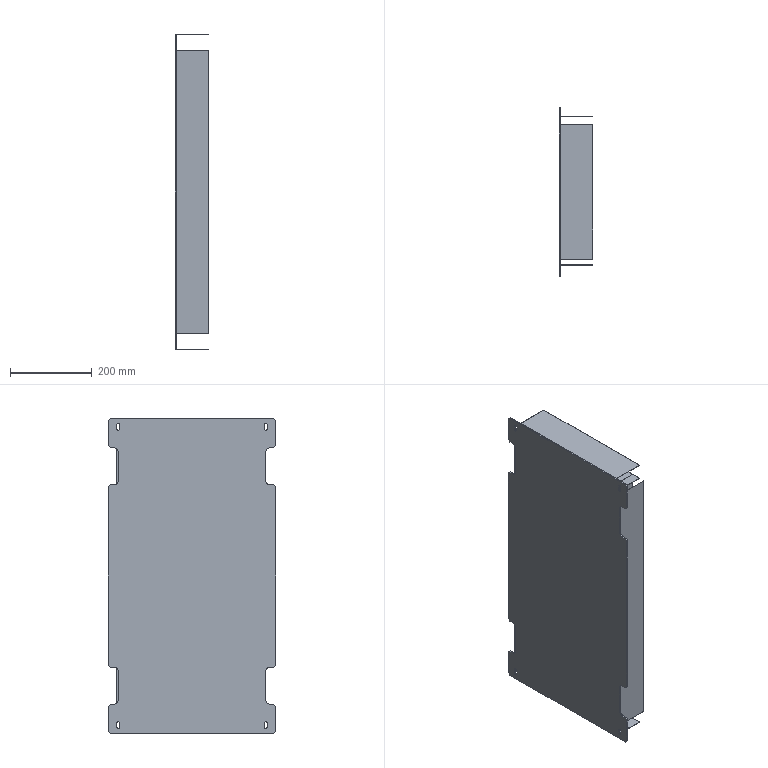Part | SolidWorks | 14 solids | 544 faces | box 83 x 410 x 770 mm | volume 1561951 mm3 | plane 294 | cylinder 250 | commonest cylinder face diameters 5.352 x78 4.5 x48 1.473 x40 4.2 x24 4.473 x24 3.473 x16